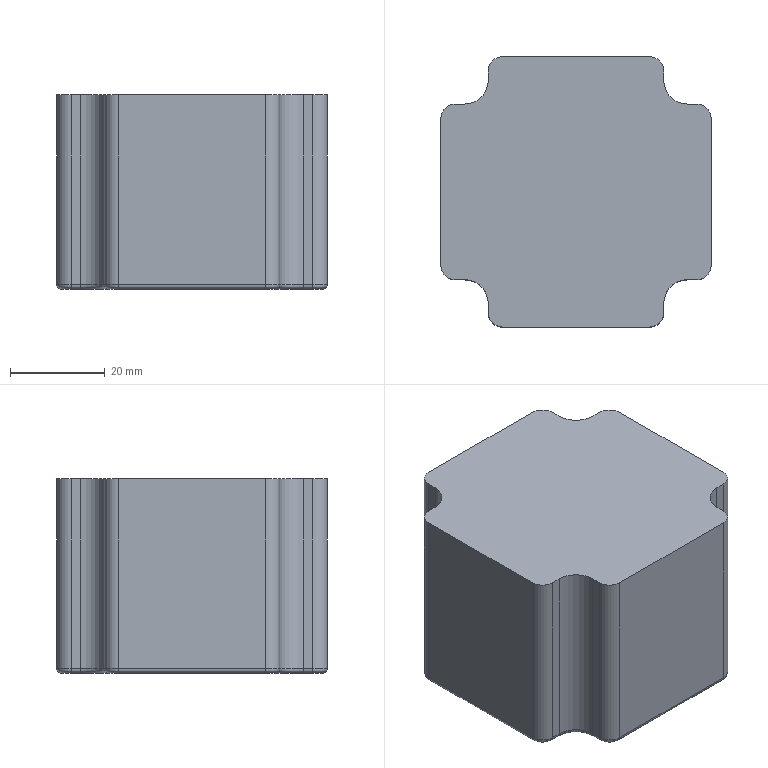Part | SolidWorks | features BaseBody 1 | 1 solid | 50 faces | box 57 x 57 x 41 mm | volume 117011 mm3 | cylinder 24 | plane 14 | torus 12 | commonest cylinder face diameters 2 x12 6 x8 10 x4
STEP:
#1=CARTESIAN_POINT('',(-18.5,23.5,41.));
#2=VERTEX_POINT('',#1);
#3=CARTESIAN_POINT('',(-18.5,23.5,1.));
#4=VERTEX_POINT('',#3);
#5=CARTESIAN_POINT('',(-18.5,23.5,41.));
#6=DIRECTION('',(0.,0.,-1.));
#7=VECTOR('',#6,1000.);
#8=LINE('',#5,#7);
#9=EDGE_CURVE('',#2,#4,#8,.T.);
#10=ORIENTED_EDGE('',*,*,#9,.T.);
#11=CARTESIAN_POINT('',(-23.5,18.5,1.));
#12=VERTEX_POINT('',#11);
#13=CARTESIAN_POINT('',(-23.5,23.5,1.));
#14=DIRECTION('',(0.,0.,-1.));
#15=DIRECTION('',(1.,0.,0.));
#16=AXIS2_PLACEMENT_3D('',#13,#14,#15);
#17=CIRCLE('',#16,5.);
#18=EDGE_CURVE('',#4,#12,#17,.T.);
#19=ORIENTED_EDGE('',*,*,#18,.T.);
#20=CARTESIAN_POINT('',(-23.5,18.5,41.));
#21=VERTEX_POINT('',#20);
#22=CARTESIAN_POINT('',(-23.5,18.5,41.));
#23=DIRECTION('',(0.,0.,-1.));
#24=VECTOR('',#23,1000.);
#25=LINE('',#22,#24);
#26=EDGE_CURVE('',#21,#12,#25,.T.);
#27=ORIENTED_EDGE('',*,*,#26,.F.);
#28=CARTESIAN_POINT('',(-23.5,23.5,41.));
#29=DIRECTION('',(0.,0.,-1.));
#30=DIRECTION('',(1.,0.,0.));
#31=AXIS2_PLACEMENT_3D('',#28,#29,#30);
#32=CIRCLE('',#31,5.);
#33=EDGE_CURVE('',#2,#21,#32,.T.);
#34=ORIENTED_EDGE('',*,*,#33,.F.);
#35=EDGE_LOOP('',(#10,#19,#27,#34));
#36=FACE_OUTER_BOUND('',#35,.T.);
#37=CARTESIAN_POINT('',(-23.5,23.5,41.));
#38=DIRECTION('',(0.,0.,-1.));
#39=DIRECTION('',(-1.,0.,0.));
#40=AXIS2_PLACEMENT_3D('',#37,#38,#39);
#41=CYLINDRICAL_SURFACE('',#40,5.);
#42=ADVANCED_FACE('',(#36),#41,.F.);
#43=ORIENTED_EDGE('',*,*,#26,.T.);
#44=CARTESIAN_POINT('',(-25.5,18.5,1.));
#45=VERTEX_POINT('',#44);
#46=CARTESIAN_POINT('',(-25.5,18.5,1.));
#47=DIRECTION('',(-1.,0.,0.));
#48=VECTOR('',#47,1000.);
#49=LINE('',#46,#48);
#50=EDGE_CURVE('',#12,#45,#49,.T.);
#51=ORIENTED_EDGE('',*,*,#50,.T.);
#52=CARTESIAN_POINT('',(-25.5,18.5,41.));
#53=VERTEX_POINT('',#52);
#54=CARTESIAN_POINT('',(-25.5,18.5,41.));
#55=DIRECTION('',(0.,0.,-1.));
#56=VECTOR('',#55,1000.);
#57=LINE('',#54,#56);
#58=EDGE_CURVE('',#53,#45,#57,.T.);
#59=ORIENTED_EDGE('',*,*,#58,.F.);
#60=CARTESIAN_POINT('',(-25.5,18.5,41.));
#61=DIRECTION('',(-1.,0.,0.));
#62=VECTOR('',#61,1000.);
#63=LINE('',#60,#62);
#64=EDGE_CURVE('',#21,#53,#63,.T.);
#65=ORIENTED_EDGE('',*,*,#64,.F.);
#66=EDGE_LOOP('',(#43,#51,#59,#65));
#67=FACE_OUTER_BOUND('',#66,.T.);
#68=CARTESIAN_POINT('',(-25.5,18.5,41.));
#69=DIRECTION('',(0.,-1.,0.));
#70=DIRECTION('',(0.,0.,-1.));
#71=AXIS2_PLACEMENT_3D('',#68,#69,#70);
#72=PLANE('',#71);
#73=ADVANCED_FACE('',(#67),#72,.F.);
#74=ORIENTED_EDGE('',*,*,#58,.T.);
#75=CARTESIAN_POINT('',(-28.5,15.5,1.));
#76=VERTEX_POINT('',#75);
#77=CARTESIAN_POINT('',(-25.5,15.5,1.));
#78=DIRECTION('',(0.,0.,1.));
#79=DIRECTION('',(1.,0.,0.));
#80=AXIS2_PLACEMENT_3D('',#77,#78,#79);
#81=CIRCLE('',#80,3.);
#82=EDGE_CURVE('',#45,#76,#81,.T.);
#83=ORIENTED_EDGE('',*,*,#82,.T.);
#84=CARTESIAN_POINT('',(-28.5,15.5,41.));
#85=VERTEX_POINT('',#84);
#86=CARTESIAN_POINT('',(-28.5,15.5,41.));
#87=DIRECTION('',(0.,0.,-1.));
#88=VECTOR('',#87,1000.);
#89=LINE('',#86,#88);
#90=EDGE_CURVE('',#85,#76,#89,.T.);
#91=ORIENTED_EDGE('',*,*,#90,.F.);
#92=CARTESIAN_POINT('',(-25.5,15.5,41.));
#93=DIRECTION('',(0.,0.,1.));
#94=DIRECTION('',(-1.,0.,0.));
#95=AXIS2_PLACEMENT_3D('',#92,#93,#94);
#96=CIRCLE('',#95,3.);
#97=EDGE_CURVE('',#53,#85,#96,.T.);
#98=ORIENTED_EDGE('',*,*,#97,.F.);
#99=EDGE_LOOP('',(#74,#83,#91,#98));
#100=FACE_OUTER_BOUND('',#99,.T.);
#101=CARTESIAN_POINT('',(-25.5,15.5,41.));
#102=DIRECTION('',(0.,0.,-1.));
#103=DIRECTION('',(-1.,0.,0.));
#104=AXIS2_PLACEMENT_3D('',#101,#102,#103);
#105=CYLINDRICAL_SURFACE('',#104,3.);
#106=ADVANCED_FACE('',(#100),#105,.T.);
#107=ORIENTED_EDGE('',*,*,#90,.T.);
#108=CARTESIAN_POINT('',(-28.5,-15.5,1.));
#109=VERTEX_POINT('',#108);
#110=CARTESIAN_POINT('',(-28.5,-15.5,1.));
#111=DIRECTION('',(0.,-1.,0.));
#112=VECTOR('',#111,1000.);
#113=LINE('',#110,#112);
#114=EDGE_CURVE('',#76,#109,#113,.T.);
#115=ORIENTED_EDGE('',*,*,#114,.T.);
#116=CARTESIAN_POINT('',(-28.5,-15.5,41.));
#117=VERTEX_POINT('',#116);
#118=CARTESIAN_POINT('',(-28.5,-15.5,41.));
#119=DIRECTION('',(0.,0.,-1.));
#120=VECTOR('',#119,1000.);
#121=LINE('',#118,#120);
#122=EDGE_CURVE('',#117,#109,#121,.T.);
#123=ORIENTED_EDGE('',*,*,#122,.F.);
#124=CARTESIAN_POINT('',(-28.5,-15.5,41.));
#125=DIRECTION('',(0.,-1.,0.));
#126=VECTOR('',#125,1000.);
#127=LINE('',#124,#126);
#128=EDGE_CURVE('',#85,#117,#127,.T.);
#129=ORIENTED_EDGE('',*,*,#128,.F.);
#130=EDGE_LOOP('',(#107,#115,#123,#129));
#131=FACE_OUTER_BOUND('',#130,.T.);
#132=CARTESIAN_POINT('',(-28.5,-15.5,41.));
#133=DIRECTION('',(1.,0.,0.));
#134=DIRECTION('',(0.,1.,0.));
#135=AXIS2_PLACEMENT_3D('',#132,#133,#134);
#136=PLANE('',#135);
#137=ADVANCED_FACE('',(#131),#136,.F.);
#138=ORIENTED_EDGE('',*,*,#122,.T.);
#139=CARTESIAN_POINT('',(-25.5,-18.5,1.));
#140=VERTEX_POINT('',#139);
#141=CARTESIAN_POINT('',(-25.5,-15.5,1.));
#142=DIRECTION('',(0.,0.,1.));
#143=DIRECTION('',(1.,0.,0.));
#144=AXIS2_PLACEMENT_3D('',#141,#142,#143);
#145=CIRCLE('',#144,3.);
#146=EDGE_CURVE('',#109,#140,#145,.T.);
#147=ORIENTED_EDGE('',*,*,#146,.T.);
#148=CARTESIAN_POINT('',(-25.5,-18.5,41.));
#149=VERTEX_POINT('',#148);
#150=CARTESIAN_POINT('',(-25.5,-18.5,41.));
#151=DIRECTION('',(0.,0.,-1.));
#152=VECTOR('',#151,1000.);
#153=LINE('',#150,#152);
#154=EDGE_CURVE('',#149,#140,#153,.T.);
#155=ORIENTED_EDGE('',*,*,#154,.F.);
#156=CARTESIAN_POINT('',(-25.5,-15.5,41.));
#157=DIRECTION('',(0.,0.,1.));
#158=DIRECTION('',(-1.,0.,0.));
#159=AXIS2_PLACEMENT_3D('',#156,#157,#158);
#160=CIRCLE('',#159,3.);
#161=EDGE_CURVE('',#117,#149,#160,.T.);
#162=ORIENTED_EDGE('',*,*,#161,.F.);
#163=EDGE_LOOP('',(#138,#147,#155,#162));
#164=FACE_OUTER_BOUND('',#163,.T.);
#165=CARTESIAN_POINT('',(-25.5,-15.5,41.));
#166=DIRECTION('',(0.,0.,-1.));
#167=DIRECTION('',(-1.,0.,0.));
#168=AXIS2_PLACEMENT_3D('',#165,#166,#167);
#169=CYLINDRICAL_SURFACE('',#168,3.);
#170=ADVANCED_FACE('',(#164),#169,.T.);
#171=ORIENTED_EDGE('',*,*,#154,.T.);
#172=CARTESIAN_POINT('',(-23.5,-18.5,1.));
#173=VERTEX_POINT('',#172);
#174=CARTESIAN_POINT('',(-25.5,-18.5,1.));
#175=DIRECTION('',(1.,0.,0.));
#176=VECTOR('',#175,1000.);
#177=LINE('',#174,#176);
#178=EDGE_CURVE('',#140,#173,#177,.T.);
#179=ORIENTED_EDGE('',*,*,#178,.T.);
#180=CARTESIAN_POINT('',(-23.5,-18.5,41.));
#181=VERTEX_POINT('',#180);
#182=CARTESIAN_POINT('',(-23.5,-18.5,41.));
#183=DIRECTION('',(0.,0.,-1.));
#184=VECTOR('',#183,1000.);
#185=LINE('',#182,#184);
#186=EDGE_CURVE('',#181,#173,#185,.T.);
#187=ORIENTED_EDGE('',*,*,#186,.F.);
#188=CARTESIAN_POINT('',(-25.5,-18.5,41.));
#189=DIRECTION('',(1.,0.,0.));
#190=VECTOR('',#189,1000.);
#191=LINE('',#188,#190);
#192=EDGE_CURVE('',#149,#181,#191,.T.);
#193=ORIENTED_EDGE('',*,*,#192,.F.);
#194=EDGE_LOOP('',(#171,#179,#187,#193));
#195=FACE_OUTER_BOUND('',#194,.T.);
#196=CARTESIAN_POINT('',(-25.5,-18.5,41.));
#197=DIRECTION('',(0.,1.,0.));
#198=DIRECTION('',(1.,0.,0.));
#199=AXIS2_PLACEMENT_3D('',#196,#197,#198);
#200=PLANE('',#199);
#201=ADVANCED_FACE('',(#195),#200,.F.);
#202=ORIENTED_EDGE('',*,*,#186,.T.);
#203=CARTESIAN_POINT('',(-18.5,-23.5,1.));
#204=VERTEX_POINT('',#203);
#205=CARTESIAN_POINT('',(-23.5,-23.5,1.));
#206=DIRECTION('',(0.,0.,-1.));
#207=DIRECTION('',(1.,0.,0.));
#208=AXIS2_PLACEMENT_3D('',#205,#206,#207);
#209=CIRCLE('',#208,5.);
#210=EDGE_CURVE('',#173,#204,#209,.T.);
#211=ORIENTED_EDGE('',*,*,#210,.T.);
#212=CARTESIAN_POINT('',(-18.5,-23.5,41.));
#213=VERTEX_POINT('',#212);
#214=CARTESIAN_POINT('',(-18.5,-23.5,41.));
#215=DIRECTION('',(0.,0.,-1.));
#216=VECTOR('',#215,1000.);
#217=LINE('',#214,#216);
#218=EDGE_CURVE('',#213,#204,#217,.T.);
#219=ORIENTED_EDGE('',*,*,#218,.F.);
#220=CARTESIAN_POINT('',(-23.5,-23.5,41.));
#221=DIRECTION('',(0.,0.,-1.));
#222=DIRECTION('',(1.,0.,0.));
#223=AXIS2_PLACEMENT_3D('',#220,#221,#222);
#224=CIRCLE('',#223,5.);
#225=EDGE_CURVE('',#181,#213,#224,.T.);
#226=ORIENTED_EDGE('',*,*,#225,.F.);
#227=EDGE_LOOP('',(#202,#211,#219,#226));
#228=FACE_OUTER_BOUND('',#227,.T.);
#229=CARTESIAN_POINT('',(-23.5,-23.5,41.));
#230=DIRECTION('',(0.,0.,-1.));
#231=DIRECTION('',(-1.,0.,0.));
#232=AXIS2_PLACEMENT_3D('',#229,#230,#231);
#233=CYLINDRICAL_SURFACE('',#232,5.);
#234=ADVANCED_FACE('',(#228),#233,.F.);
#235=ORIENTED_EDGE('',*,*,#218,.T.);
#236=CARTESIAN_POINT('',(-18.5,-25.5,1.));
#237=VERTEX_POINT('',#236);
#238=CARTESIAN_POINT('',(-18.5,-25.5,1.));
#239=DIRECTION('',(0.,-1.,0.));
#240=VECTOR('',#239,1000.);
#241=LINE('',#238,#240);
#242=EDGE_CURVE('',#204,#237,#241,.T.);
#243=ORIENTED_EDGE('',*,*,#242,.T.);
#244=CARTESIAN_POINT('',(-18.5,-25.5,41.));
#245=VERTEX_POINT('',#244);
#246=CARTESIAN_POINT('',(-18.5,-25.5,41.));
#247=DIRECTION('',(0.,0.,-1.));
#248=VECTOR('',#247,1000.);
#249=LINE('',#246,#248);
#250=EDGE_CURVE('',#245,#237,#249,.T.);
#251=ORIENTED_EDGE('',*,*,#250,.F.);
#252=CARTESIAN_POINT('',(-18.5,-25.5,41.));
#253=DIRECTION('',(0.,-1.,0.));
#254=VECTOR('',#253,1000.);
#255=LINE('',#252,#254);
#256=EDGE_CURVE('',#213,#245,#255,.T.);
#257=ORIENTED_EDGE('',*,*,#256,.F.);
#258=EDGE_LOOP('',(#235,#243,#251,#257));
#259=FACE_OUTER_BOUND('',#258,.T.);
#260=CARTESIAN_POINT('',(-18.5,-25.5,41.));
#261=DIRECTION('',(1.,0.,0.));
#262=DIRECTION('',(0.,1.,0.));
#263=AXIS2_PLACEMENT_3D('',#260,#261,#262);
#264=PLANE('',#263);
#265=ADVANCED_FACE('',(#259),#264,.F.);
#266=ORIENTED_EDGE('',*,*,#250,.T.);
#267=CARTESIAN_POINT('',(-15.5,-28.5,1.));
#268=VERTEX_POINT('',#267);
#269=CARTESIAN_POINT('',(-15.5,-25.5,1.));
#270=DIRECTION('',(0.,0.,1.));
#271=DIRECTION('',(1.,0.,0.));
#272=AXIS2_PLACEMENT_3D('',#269,#270,#271);
#273=CIRCLE('',#272,3.);
#274=EDGE_CURVE('',#237,#268,#273,.T.);
#275=ORIENTED_EDGE('',*,*,#274,.T.);
#276=CARTESIAN_POINT('',(-15.5,-28.5,41.));
#277=VERTEX_POINT('',#276);
#278=CARTESIAN_POINT('',(-15.5,-28.5,41.));
#279=DIRECTION('',(0.,0.,-1.));
#280=VECTOR('',#279,1000.);
#281=LINE('',#278,#280);
#282=EDGE_CURVE('',#277,#268,#281,.T.);
#283=ORIENTED_EDGE('',*,*,#282,.F.);
#284=CARTESIAN_POINT('',(-15.5,-25.5,41.));
#285=DIRECTION('',(0.,0.,1.));
#286=DIRECTION('',(-1.,0.,0.));
#287=AXIS2_PLACEMENT_3D('',#284,#285,#286);
#288=CIRCLE('',#287,3.);
#289=EDGE_CURVE('',#245,#277,#288,.T.);
#290=ORIENTED_EDGE('',*,*,#289,.F.);
#291=EDGE_LOOP('',(#266,#275,#283,#290));
#292=FACE_OUTER_BOUND('',#291,.T.);
#293=CARTESIAN_POINT('',(-15.5,-25.5,41.));
#294=DIRECTION('',(0.,0.,-1.));
#295=DIRECTION('',(-1.,0.,0.));
#296=AXIS2_PLACEMENT_3D('',#293,#294,#295);
#297=CYLINDRICAL_SURFACE('',#296,3.);
#298=ADVANCED_FACE('',(#292),#297,.T.);
#299=ORIENTED_EDGE('',*,*,#282,.T.);
#300=CARTESIAN_POINT('',(15.5,-28.5,1.));
#301=VERTEX_POINT('',#300);
#302=CARTESIAN_POINT('',(-15.5,-28.5,1.));
#303=DIRECTION('',(1.,0.,0.));
#304=VECTOR('',#303,1000.);
#305=LINE('',#302,#304);
#306=EDGE_CURVE('',#268,#301,#305,.T.);
#307=ORIENTED_EDGE('',*,*,#306,.T.);
#308=CARTESIAN_POINT('',(15.5,-28.5,41.));
#309=VERTEX_POINT('',#308);
#310=CARTESIAN_POINT('',(15.5,-28.5,41.));
#311=DIRECTION('',(0.,0.,-1.));
#312=VECTOR('',#311,1000.);
#313=LINE('',#310,#312);
#314=EDGE_CURVE('',#309,#301,#313,.T.);
#315=ORIENTED_EDGE('',*,*,#314,.F.);
#316=CARTESIAN_POINT('',(-15.5,-28.5,41.));
#317=DIRECTION('',(1.,0.,0.));
#318=VECTOR('',#317,1000.);
#319=LINE('',#316,#318);
#320=EDGE_CURVE('',#277,#309,#319,.T.);
#321=ORIENTED_EDGE('',*,*,#320,.F.);
#322=EDGE_LOOP('',(#299,#307,#315,#321));
#323=FACE_OUTER_BOUND('',#322,.T.);
#324=CARTESIAN_POINT('',(-15.5,-28.5,41.));
#325=DIRECTION('',(0.,1.,0.));
#326=DIRECTION('',(1.,0.,0.));
#327=AXIS2_PLACEMENT_3D('',#324,#325,#326);
#328=PLANE('',#327);
#329=ADVANCED_FACE('',(#323),#328,.F.);
#330=ORIENTED_EDGE('',*,*,#314,.T.);
#331=CARTESIAN_POINT('',(18.5,-25.5,1.));
#332=VERTEX_POINT('',#331);
#333=CARTESIAN_POINT('',(15.5,-25.5,1.));
#334=DIRECTION('',(0.,0.,1.));
#335=DIRECTION('',(1.,0.,0.));
#336=AXIS2_PLACEMENT_3D('',#333,#334,#335);
#337=CIRCLE('',#336,3.);
#338=EDGE_CURVE('',#301,#332,#337,.T.);
#339=ORIENTED_EDGE('',*,*,#338,.T.);
#340=CARTESIAN_POINT('',(18.5,-25.5,41.));
#341=VERTEX_POINT('',#340);
#342=CARTESIAN_POINT('',(18.5,-25.5,41.));
#343=DIRECTION('',(0.,0.,-1.));
#344=VECTOR('',#343,1000.);
#345=LINE('',#342,#344);
#346=EDGE_CURVE('',#341,#332,#345,.T.);
#347=ORIENTED_EDGE('',*,*,#346,.F.);
#348=CARTESIAN_POINT('',(15.5,-25.5,41.));
#349=DIRECTION('',(0.,0.,1.));
#350=DIRECTION('',(1.,0.,0.));
#351=AXIS2_PLACEMENT_3D('',#348,#349,#350);
#352=CIRCLE('',#351,3.);
#353=EDGE_CURVE('',#309,#341,#352,.T.);
#354=ORIENTED_EDGE('',*,*,#353,.F.);
#355=EDGE_LOOP('',(#330,#339,#347,#354));
#356=FACE_OUTER_BOUND('',#355,.T.);
#357=CARTESIAN_POINT('',(15.5,-25.5,41.));
#358=DIRECTION('',(0.,0.,-1.));
#359=DIRECTION('',(-1.,0.,0.));
#360=AXIS2_PLACEMENT_3D('',#357,#358,#359);
#361=CYLINDRICAL_SURFACE('',#360,3.);
#362=ADVANCED_FACE('',(#356),#361,.T.);
#363=ORIENTED_EDGE('',*,*,#346,.T.);
#364=CARTESIAN_POINT('',(18.5,-23.5,1.));
#365=VERTEX_POINT('',#364);
#366=CARTESIAN_POINT('',(18.5,-25.5,1.));
#367=DIRECTION('',(0.,1.,0.));
#368=VECTOR('',#367,1000.);
#369=LINE('',#366,#368);
#370=EDGE_CURVE('',#332,#365,#369,.T.);
#371=ORIENTED_EDGE('',*,*,#370,.T.);
#372=CARTESIAN_POINT('',(18.5,-23.5,41.));
#373=VERTEX_POINT('',#372);
#374=CARTESIAN_POINT('',(18.5,-23.5,41.));
#375=DIRECTION('',(0.,0.,-1.));
#376=VECTOR('',#375,1000.);
#377=LINE('',#374,#376);
#378=EDGE_CURVE('',#373,#365,#377,.T.);
#379=ORIENTED_EDGE('',*,*,#378,.F.);
#380=CARTESIAN_POINT('',(18.5,-25.5,41.));
#381=DIRECTION('',(0.,1.,0.));
#382=VECTOR('',#381,1000.);
#383=LINE('',#380,#382);
#384=EDGE_CURVE('',#341,#373,#383,.T.);
#385=ORIENTED_EDGE('',*,*,#384,.F.);
#386=EDGE_LOOP('',(#363,#371,#379,#385));
#387=FACE_OUTER_BOUND('',#386,.T.);
#388=CARTESIAN_POINT('',(18.5,-25.5,41.));
#389=DIRECTION('',(-1.,0.,0.));
#390=DIRECTION('',(0.,0.,1.));
#391=AXIS2_PLACEMENT_3D('',#388,#389,#390);
#392=PLANE('',#391);
#393=ADVANCED_FACE('',(#387),#392,.F.);
#394=ORIENTED_EDGE('',*,*,#378,.T.);
#395=CARTESIAN_POINT('',(23.5,-18.5,1.));
#396=VERTEX_POINT('',#395);
#397=CARTESIAN_POINT('',(23.5,-23.5,1.));
#398=DIRECTION('',(0.,0.,-1.));
#399=DIRECTION('',(1.,0.,0.));
#400=AXIS2_PLACEMENT_3D('',#397,#398,#399);
#401=CIRCLE('',#400,5.);
#402=EDGE_CURVE('',#365,#396,#401,.T.);
#403=ORIENTED_EDGE('',*,*,#402,.T.);
#404=CARTESIAN_POINT('',(23.5,-18.5,41.));
#405=VERTEX_POINT('',#404);
#406=CARTESIAN_POINT('',(23.5,-18.5,41.));
#407=DIRECTION('',(0.,0.,-1.));
#408=VECTOR('',#407,1000.);
#409=LINE('',#406,#408);
#410=EDGE_CURVE('',#405,#396,#409,.T.);
#411=ORIENTED_EDGE('',*,*,#410,.F.);
#412=CARTESIAN_POINT('',(23.5,-23.5,41.));
#413=DIRECTION('',(0.,0.,-1.));
#414=DIRECTION('',(1.,0.,0.));
#415=AXIS2_PLACEMENT_3D('',#412,#413,#414);
#416=CIRCLE('',#415,5.);
#417=EDGE_CURVE('',#373,#405,#416,.T.);
#418=ORIENTED_EDGE('',*,*,#417,.F.);
#419=EDGE_LOOP('',(#394,#403,#411,#418));
#420=FACE_OUTER_BOUND('',#419,.T.);
#421=CARTESIAN_POINT('',(23.5,-23.5,41.));
#422=DIRECTION('',(0.,0.,-1.));
#423=DIRECTION('',(-1.,0.,0.));
#424=AXIS2_PLACEMENT_3D('',#421,#422,#423);
#425=CYLINDRICAL_SURFACE('',#424,5.);
#426=ADVANCED_FACE('',(#420),#425,.F.);
#427=ORIENTED_EDGE('',*,*,#410,.T.);
#428=CARTESIAN_POINT('',(25.5,-18.5,1.));
#429=VERTEX_POINT('',#428);
#430=CARTESIAN_POINT('',(25.5,-18.5,1.));
#431=DIRECTION('',(1.,0.,0.));
#432=VECTOR('',#431,1000.);
#433=LINE('',#430,#432);
#434=EDGE_CURVE('',#396,#429,#433,.T.);
#435=ORIENTED_EDGE('',*,*,#434,.T.);
#436=CARTESIAN_POINT('',(25.5,-18.5,41.));
#437=VERTEX_POINT('',#436);
#438=CARTESIAN_POINT('',(25.5,-18.5,41.));
#439=DIRECTION('',(0.,0.,-1.));
#440=VECTOR('',#439,1000.);
#441=LINE('',#438,#440);
#442=EDGE_CURVE('',#437,#429,#441,.T.);
#443=ORIENTED_EDGE('',*,*,#442,.F.);
#444=CARTESIAN_POINT('',(25.5,-18.5,41.));
#445=DIRECTION('',(1.,0.,0.));
#446=VECTOR('',#445,1000.);
#447=LINE('',#444,#446);
#448=EDGE_CURVE('',#405,#437,#447,.T.);
#449=ORIENTED_EDGE('',*,*,#448,.F.);
#450=EDGE_LOOP('',(#427,#435,#443,#449));
#451=FACE_OUTER_BOUND('',#450,.T.);
#452=CARTESIAN_POINT('',(25.5,-18.5,41.));
#453=DIRECTION('',(0.,1.,0.));
#454=DIRECTION('',(1.,0.,0.));
#455=AXIS2_PLACEMENT_3D('',#452,#453,#454);
#456=PLANE('',#455);
#457=ADVANCED_FACE('',(#451),#456,.F.);
#458=ORIENTED_EDGE('',*,*,#442,.T.);
#459=CARTESIAN_POINT('',(28.5,-15.5,1.));
#460=VERTEX_POINT('',#459);
#461=CARTESIAN_POINT('',(25.5,-15.5,1.));
#462=DIRECTION('',(0.,0.,1.));
#463=DIRECTION('',(1.,0.,0.));
#464=AXIS2_PLACEMENT_3D('',#461,#462,#463);
#465=CIRCLE('',#464,3.);
#466=EDGE_CURVE('',#429,#460,#465,.T.);
#467=ORIENTED_EDGE('',*,*,#466,.T.);
#468=CARTESIAN_POINT('',(28.5,-15.5,41.));
#469=VERTEX_POINT('',#468);
#470=CARTESIAN_POINT('',(28.5,-15.5,41.));
#471=DIRECTION('',(0.,0.,-1.));
#472=VECTOR('',#471,1000.);
#473=LINE('',#470,#472);
#474=EDGE_CURVE('',#469,#460,#473,.T.);
#475=ORIENTED_EDGE('',*,*,#474,.F.);
#476=CARTESIAN_POINT('',(25.5,-15.5,41.));
#477=DIRECTION('',(0.,0.,1.));
#478=DIRECTION('',(-1.,0.,0.));
#479=AXIS2_PLACEMENT_3D('',#476,#477,#478);
#480=CIRCLE('',#479,3.);
#481=EDGE_CURVE('',#437,#469,#480,.T.);
#482=ORIENTED_EDGE('',*,*,#481,.F.);
#483=EDGE_LOOP('',(#458,#467,#475,#482));
#484=FACE_OUTER_BOUND('',#483,.T.);
#485=CARTESIAN_POINT('',(25.5,-15.5,41.));
#486=DIRECTION('',(0.,0.,-1.));
#487=DIRECTION('',(-1.,0.,0.));
#488=AXIS2_PLACEMENT_3D('',#485,#486,#487);
#489=CYLINDRICAL_SURFACE('',#488,3.);
#490=ADVANCED_FACE('',(#484),#489,.T.);
#491=ORIENTED_EDGE('',*,*,#474,.T.);
#492=CARTESIAN_POINT('',(28.5,15.5,1.));
#493=VERTEX_POINT('',#492);
#494=CARTESIAN_POINT('',(28.5,-15.5,1.));
#495=DIRECTION('',(0.,1.,0.));
#496=VECTOR('',#495,1000.);
#497=LINE('',#494,#496);
#498=EDGE_CURVE('',#460,#493,#497,.T.);
#499=ORIENTED_EDGE('',*,*,#498,.T.);
#500=CARTESIAN_POINT('',(28.5,15.5,41.));
#501=VERTEX_POINT('',#500);
#502=CARTESIAN_POINT('',(28.5,15.5,41.));
#503=DIRECTION('',(0.,0.,-1.));
#504=VECTOR('',#503,1000.);
#505=LINE('',#502,#504);
#506=EDGE_CURVE('',#501,#493,#505,.T.);
#507=ORIENTED_EDGE('',*,*,#506,.F.);
#508=CARTESIAN_POINT('',(28.5,-15.5,41.));
#509=DIRECTION('',(0.,1.,0.));
#510=VECTOR('',#509,1000.);
#511=LINE('',#508,#510);
#512=EDGE_CURVE('',#469,#501,#511,.T.);
#513=ORIENTED_EDGE('',*,*,#512,.F.);
#514=EDGE_LOOP('',(#491,#499,#507,#513));
#515=FACE_OUTER_BOUND('',#514,.T.);
#516=CARTESIAN_POINT('',(28.5,-15.5,41.));
#517=DIRECTION('',(-1.,0.,0.));
#518=DIRECTION('',(0.,0.,1.));
#519=AXIS2_PLACEMENT_3D('',#516,#517,#518);
#520=PLANE('',#519);
#521=ADVANCED_FACE('',(#515),#520,.F.);
#522=ORIENTED_EDGE('',*,*,#506,.T.);
#523=CARTESIAN_POINT('',(25.5,18.5,1.));
#524=VERTEX_POINT('',#523);
#525=CARTESIAN_POINT('',(25.5,15.5,1.));
#526=DIRECTION('',(0.,0.,1.));
#527=DIRECTION('',(1.,0.,0.));
#528=AXIS2_PLACEMENT_3D('',#525,#526,#527);
#529=CIRCLE('',#528,3.);
#530=EDGE_CURVE('',#493,#524,#529,.T.);
#531=ORIENTED_EDGE('',*,*,#530,.T.);
#532=CARTESIAN_POINT('',(25.5,18.5,41.));
#533=VERTEX_POINT('',#532);
#534=CARTESIAN_POINT('',(25.5,18.5,41.));
#535=DIRECTION('',(0.,0.,-1.));
#536=VECTOR('',#535,1000.);
#537=LINE('',#534,#536);
#538=EDGE_CURVE('',#533,#524,#537,.T.);
#539=ORIENTED_EDGE('',*,*,#538,.F.);
#540=CARTESIAN_POINT('',(25.5,15.5,41.));
#541=DIRECTION('',(0.,0.,1.));
#542=DIRECTION('',(1.,0.,0.));
#543=AXIS2_PLACEMENT_3D('',#540,#541,#542);
#544=CIRCLE('',#543,3.);
#545=EDGE_CURVE('',#501,#533,#544,.T.);
#546=ORIENTED_EDGE('',*,*,#545,.F.);
#547=EDGE_LOOP('',(#522,#531,#539,#546));
#548=FACE_OUTER_BOUND('',#547,.T.);
#549=CARTESIAN_POINT('',(25.5,15.5,41.));
#550=DIRECTION('',(0.,0.,-1.));
#551=DIRECTION('',(-1.,0.,0.));
#552=AXIS2_PLACEMENT_3D('',#549,#550,#551);
#553=CYLINDRICAL_SURFACE('',#552,3.);
#554=ADVANCED_FACE('',(#548),#553,.T.);
#555=ORIENTED_EDGE('',*,*,#538,.T.);
#556=CARTESIAN_POINT('',(23.5,18.5,1.));
#557=VERTEX_POINT('',#556);
#558=CARTESIAN_POINT('',(25.5,18.5,1.));
#559=DIRECTION('',(-1.,0.,0.));
#560=VECTOR('',#559,1000.);
#561=LINE('',#558,#560);
#562=EDGE_CURVE('',#524,#557,#561,.T.);
#563=ORIENTED_EDGE('',*,*,#562,.T.);
#564=CARTESIAN_POINT('',(23.5,18.5,41.));
#565=VERTEX_POINT('',#564);
#566=CARTESIAN_POINT('',(23.5,18.5,41.));
#567=DIRECTION('',(0.,0.,-1.));
#568=VECTOR('',#567,1000.);
#569=LINE('',#566,#568);
#570=EDGE_CURVE('',#565,#557,#569,.T.);
#571=ORIENTED_EDGE('',*,*,#570,.F.);
#572=CARTESIAN_POINT('',(25.5,18.5,41.));
#573=DIRECTION('',(-1.,0.,0.));
#574=VECTOR('',#573,1000.);
#575=LINE('',#572,#574);
#576=EDGE_CURVE('',#533,#565,#575,.T.);
#577=ORIENTED_EDGE('',*,*,#576,.F.);
#578=EDGE_LOOP('',(#555,#563,#571,#577));
#579=FACE_OUTER_BOUND('',#578,.T.);
#580=CARTESIAN_POINT('',(25.5,18.5,41.));
#581=DIRECTION('',(0.,-1.,0.));
#582=DIRECTION('',(0.,0.,-1.));
#583=AXIS2_PLACEMENT_3D('',#580,#581,#582);
#584=PLANE('',#583);
#585=ADVANCED_FACE('',(#579),#584,.F.);
#586=ORIENTED_EDGE('',*,*,#570,.T.);
#587=CARTESIAN_POINT('',(18.5,23.5,1.));
#588=VERTEX_POINT('',#587);
#589=CARTESIAN_POINT('',(23.5,23.5,1.));
#590=DIRECTION('',(0.,0.,-1.));
#591=DIRECTION('',(1.,0.,0.));
#592=AXIS2_PLACEMENT_3D('',#589,#590,#591);
#593=CIRCLE('',#592,5.);
#594=EDGE_CURVE('',#557,#588,#593,.T.);
#595=ORIENTED_EDGE('',*,*,#594,.T.);
#596=CARTESIAN_POINT('',(18.5,23.5,41.));
#597=VERTEX_POINT('',#596);
#598=CARTESIAN_POINT('',(18.5,23.5,41.));
#599=DIRECTION('',(0.,0.,-1.));
#600=VECTOR('',#599,1000.);
#601=LINE('',#598,#600);
#602=EDGE_CURVE('',#597,#588,#601,.T.);
#603=ORIENTED_EDGE('',*,*,#602,.F.);
#604=CARTESIAN_POINT('',(23.5,23.5,41.));
#605=DIRECTION('',(0.,0.,-1.));
#606=DIRECTION('',(1.,0.,0.));
#607=AXIS2_PLACEMENT_3D('',#604,#605,#606);
#608=CIRCLE('',#607,5.);
#609=EDGE_CURVE('',#565,#597,#608,.T.);
#610=ORIENTED_EDGE('',*,*,#609,.F.);
#611=EDGE_LOOP('',(#586,#595,#603,#610));
#612=FACE_OUTER_BOUND('',#611,.T.);
#613=CARTESIAN_POINT('',(23.5,23.5,41.));
#614=DIRECTION('',(0.,0.,-1.));
#615=DIRECTION('',(-1.,0.,0.));
#616=AXIS2_PLACEMENT_3D('',#613,#614,#615);
#617=CYLINDRICAL_SURFACE('',#616,5.);
#618=ADVANCED_FACE('',(#612),#617,.F.);
#619=ORIENTED_EDGE('',*,*,#602,.T.);
#620=CARTESIAN_POINT('',(18.5,25.5,1.));
#621=VERTEX_POINT('',#620);
#622=CARTESIAN_POINT('',(18.5,25.5,1.));
#623=DIRECTION('',(0.,1.,0.));
#624=VECTOR('',#623,1000.);
#625=LINE('',#622,#624);
#626=EDGE_CURVE('',#588,#621,#625,.T.);
#627=ORIENTED_EDGE('',*,*,#626,.T.);
#628=CARTESIAN_POINT('',(18.5,25.5,41.));
#629=VERTEX_POINT('',#628);
#630=CARTESIAN_POINT('',(18.5,25.5,41.));
#631=DIRECTION('',(0.,0.,-1.));
#632=VECTOR('',#631,1000.);
#633=LINE('',#630,#632);
#634=EDGE_CURVE('',#629,#621,#633,.T.);
#635=ORIENTED_EDGE('',*,*,#634,.F.);
#636=CARTESIAN_POINT('',(18.5,25.5,41.));
#637=DIRECTION('',(0.,1.,0.));
#638=VECTOR('',#637,1000.);
#639=LINE('',#636,#638);
#640=EDGE_CURVE('',#597,#629,#639,.T.);
#641=ORIENTED_EDGE('',*,*,#640,.F.);
#642=EDGE_LOOP('',(#619,#627,#635,#641));
#643=FACE_OUTER_BOUND('',#642,.T.);
#644=CARTESIAN_POINT('',(18.5,25.5,41.));
#645=DIRECTION('',(-1.,0.,0.));
#646=DIRECTION('',(0.,1.,0.));
#647=AXIS2_PLACEMENT_3D('',#644,#645,#646);
#648=PLANE('',#647);
#649=ADVANCED_FACE('',(#643),#648,.F.);
#650=ORIENTED_EDGE('',*,*,#634,.T.);
#651=CARTESIAN_POINT('',(15.5,28.5,1.));
#652=VERTEX_POINT('',#651);
#653=CARTESIAN_POINT('',(15.5,25.5,1.));
#654=DIRECTION('',(0.,0.,1.));
#655=DIRECTION('',(1.,0.,0.));
#656=AXIS2_PLACEMENT_3D('',#653,#654,#655);
#657=CIRCLE('',#656,3.);
#658=EDGE_CURVE('',#621,#652,#657,.T.);
#659=ORIENTED_EDGE('',*,*,#658,.T.);
#660=CARTESIAN_POINT('',(15.5,28.5,41.));
#661=VERTEX_POINT('',#660);
#662=CARTESIAN_POINT('',(15.5,28.5,41.));
#663=DIRECTION('',(0.,0.,-1.));
#664=VECTOR('',#663,1000.);
#665=LINE('',#662,#664);
#666=EDGE_CURVE('',#661,#652,#665,.T.);
#667=ORIENTED_EDGE('',*,*,#666,.F.);
#668=CARTESIAN_POINT('',(15.5,25.5,41.));
#669=DIRECTION('',(0.,0.,1.));
#670=DIRECTION('',(1.,0.,0.));
#671=AXIS2_PLACEMENT_3D('',#668,#669,#670);
#672=CIRCLE('',#671,3.);
#673=EDGE_CURVE('',#629,#661,#672,.T.);
#674=ORIENTED_EDGE('',*,*,#673,.F.);
#675=EDGE_LOOP('',(#650,#659,#667,#674));
#676=FACE_OUTER_BOUND('',#675,.T.);
#677=CARTESIAN_POINT('',(15.5,25.5,41.));
#678=DIRECTION('',(0.,0.,-1.));
#679=DIRECTION('',(-1.,0.,0.));
#680=AXIS2_PLACEMENT_3D('',#677,#678,#679);
#681=CYLINDRICAL_SURFACE('',#680,3.);
#682=ADVANCED_FACE('',(#676),#681,.T.);
#683=ORIENTED_EDGE('',*,*,#666,.T.);
#684=CARTESIAN_POINT('',(-15.5,28.5,1.));
#685=VERTEX_POINT('',#684);
#686=CARTESIAN_POINT('',(-15.5,28.5,1.));
#687=DIRECTION('',(-1.,0.,0.));
#688=VECTOR('',#687,1000.);
#689=LINE('',#686,#688);
#690=EDGE_CURVE('',#652,#685,#689,.T.);
#691=ORIENTED_EDGE('',*,*,#690,.T.);
#692=CARTESIAN_POINT('',(-15.5,28.5,41.));
#693=VERTEX_POINT('',#692);
#694=CARTESIAN_POINT('',(-15.5,28.5,41.));
#695=DIRECTION('',(0.,0.,-1.));
#696=VECTOR('',#695,1000.);
#697=LINE('',#694,#696);
#698=EDGE_CURVE('',#693,#685,#697,.T.);
#699=ORIENTED_EDGE('',*,*,#698,.F.);
#700=CARTESIAN_POINT('',(-15.5,28.5,41.));
#701=DIRECTION('',(-1.,0.,0.));
#702=VECTOR('',#701,1000.);
#703=LINE('',#700,#702);
#704=EDGE_CURVE('',#661,#693,#703,.T.);
#705=ORIENTED_EDGE('',*,*,#704,.F.);
#706=EDGE_LOOP('',(#683,#691,#699,#705));
#707=FACE_OUTER_BOUND('',#706,.T.);
#708=CARTESIAN_POINT('',(-15.5,28.5,41.));
#709=DIRECTION('',(0.,-1.,0.));
#710=DIRECTION('',(0.,0.,-1.));
#711=AXIS2_PLACEMENT_3D('',#708,#709,#710);
#712=PLANE('',#711);
#713=ADVANCED_FACE('',(#707),#712,.F.);
#714=ORIENTED_EDGE('',*,*,#698,.T.);
#715=CARTESIAN_POINT('',(-18.5,25.5,1.));
#716=VERTEX_POINT('',#715);
#717=CARTESIAN_POINT('',(-15.5,25.5,1.));
#718=DIRECTION('',(0.,0.,1.));
#719=DIRECTION('',(1.,0.,0.));
#720=AXIS2_PLACEMENT_3D('',#717,#718,#719);
#721=CIRCLE('',#720,3.);
#722=EDGE_CURVE('',#685,#716,#721,.T.);
#723=ORIENTED_EDGE('',*,*,#722,.T.);
#724=CARTESIAN_POINT('',(-18.5,25.5,41.));
#725=VERTEX_POINT('',#724);
#726=CARTESIAN_POINT('',(-18.5,25.5,41.));
#727=DIRECTION('',(0.,0.,-1.));
#728=VECTOR('',#727,1000.);
#729=LINE('',#726,#728);
#730=EDGE_CURVE('',#725,#716,#729,.T.);
#731=ORIENTED_EDGE('',*,*,#730,.F.);
#732=CARTESIAN_POINT('',(-15.5,25.5,41.));
#733=DIRECTION('',(0.,0.,1.));
#734=DIRECTION('',(-1.,0.,0.));
#735=AXIS2_PLACEMENT_3D('',#732,#733,#734);
#736=CIRCLE('',#735,3.);
#737=EDGE_CURVE('',#693,#725,#736,.T.);
#738=ORIENTED_EDGE('',*,*,#737,.F.);
#739=EDGE_LOOP('',(#714,#723,#731,#738));
#740=FACE_OUTER_BOUND('',#739,.T.);
#741=CARTESIAN_POINT('',(-15.5,25.5,41.));
#742=DIRECTION('',(0.,0.,-1.));
#743=DIRECTION('',(-1.,0.,0.));
#744=AXIS2_PLACEMENT_3D('',#741,#742,#743);
#745=CYLINDRICAL_SURFACE('',#744,3.);
#746=ADVANCED_FACE('',(#740),#745,.T.);
#747=ORIENTED_EDGE('',*,*,#730,.T.);
#748=CARTESIAN_POINT('',(-18.5,25.5,1.));
#749=DIRECTION('',(0.,-1.,0.));
#750=VECTOR('',#749,1000.);
#751=LINE('',#748,#750);
#752=EDGE_CURVE('',#716,#4,#751,.T.);
#753=ORIENTED_EDGE('',*,*,#752,.T.);
#754=ORIENTED_EDGE('',*,*,#9,.F.);
#755=CARTESIAN_POINT('',(-18.5,25.5,41.));
#756=DIRECTION('',(0.,-1.,0.));
#757=VECTOR('',#756,1000.);
#758=LINE('',#755,#757);
#759=EDGE_CURVE('',#725,#2,#758,.T.);
#760=ORIENTED_EDGE('',*,*,#759,.F.);
#761=EDGE_LOOP('',(#747,#753,#754,#760));
#762=FACE_OUTER_BOUND('',#761,.T.);
#763=CARTESIAN_POINT('',(-18.5,25.5,41.));
#764=DIRECTION('',(1.,0.,0.));
#765=DIRECTION('',(0.,-1.,0.));
#766=AXIS2_PLACEMENT_3D('',#763,#764,#765);
#767=PLANE('',#766);
#768=ADVANCED_FACE('',(#762),#767,.F.);
#769=ORIENTED_EDGE('',*,*,#33,.T.);
#770=ORIENTED_EDGE('',*,*,#64,.T.);
#771=ORIENTED_EDGE('',*,*,#97,.T.);
#772=ORIENTED_EDGE('',*,*,#128,.T.);
#773=ORIENTED_EDGE('',*,*,#161,.T.);
#774=ORIENTED_EDGE('',*,*,#192,.T.);
#775=ORIENTED_EDGE('',*,*,#225,.T.);
#776=ORIENTED_EDGE('',*,*,#256,.T.);
#777=ORIENTED_EDGE('',*,*,#289,.T.);
#778=ORIENTED_EDGE('',*,*,#320,.T.);
#779=ORIENTED_EDGE('',*,*,#353,.T.);
#780=ORIENTED_EDGE('',*,*,#384,.T.);
#781=ORIENTED_EDGE('',*,*,#417,.T.);
#782=ORIENTED_EDGE('',*,*,#448,.T.);
#783=ORIENTED_EDGE('',*,*,#481,.T.);
#784=ORIENTED_EDGE('',*,*,#512,.T.);
#785=ORIENTED_EDGE('',*,*,#545,.T.);
#786=ORIENTED_EDGE('',*,*,#576,.T.);
#787=ORIENTED_EDGE('',*,*,#609,.T.);
#788=ORIENTED_EDGE('',*,*,#640,.T.);
#789=ORIENTED_EDGE('',*,*,#673,.T.);
#790=ORIENTED_EDGE('',*,*,#704,.T.);
#791=ORIENTED_EDGE('',*,*,#737,.T.);
#792=ORIENTED_EDGE('',*,*,#759,.T.);
#793=EDGE_LOOP('',(#769,#770,#771,#772,#773,#774,#775,#776,#777,#778,#779,#780,#781,#782,#783,#784,#785,#786,#787,#788,#789,#790,#791,#792));
#794=FACE_OUTER_BOUND('',#793,.T.);
#795=CARTESIAN_POINT('',(-23.5,23.5,41.));
#796=DIRECTION('',(0.,0.,1.));
#797=DIRECTION('',(1.,0.,0.));
#798=AXIS2_PLACEMENT_3D('',#795,#796,#797);
#799=PLANE('',#798);
#800=ADVANCED_FACE('',(#794),#799,.T.);
#801=CARTESIAN_POINT('',(-27.5,15.5,0.));
#802=VERTEX_POINT('',#801);
#803=CARTESIAN_POINT('',(-25.5,17.5,0.));
#804=VERTEX_POINT('',#803);
#805=CARTESIAN_POINT('',(-25.5,15.5,0.));
#806=DIRECTION('',(0.,0.,-1.));
#807=DIRECTION('',(1.,0.,0.));
#808=AXIS2_PLACEMENT_3D('',#805,#806,#807);
#809=CIRCLE('',#808,2.);
#810=EDGE_CURVE('',#802,#804,#809,.T.);
#811=ORIENTED_EDGE('',*,*,#810,.T.);
#812=CARTESIAN_POINT('',(-23.5,17.5,0.));
#813=VERTEX_POINT('',#812);
#814=CARTESIAN_POINT('',(-23.5,17.5,0.));
#815=DIRECTION('',(1.,0.,0.));
#816=VECTOR('',#815,1000.);
#817=LINE('',#814,#816);
#818=EDGE_CURVE('',#804,#813,#817,.T.);
#819=ORIENTED_EDGE('',*,*,#818,.T.);
#820=CARTESIAN_POINT('',(-17.5,23.5,0.));
#821=VERTEX_POINT('',#820);
#822=CARTESIAN_POINT('',(-23.5,23.5,0.));
#823=DIRECTION('',(0.,0.,1.));
#824=DIRECTION('',(1.,0.,0.));
#825=AXIS2_PLACEMENT_3D('',#822,#823,#824);
#826=CIRCLE('',#825,6.);
#827=EDGE_CURVE('',#813,#821,#826,.T.);
#828=ORIENTED_EDGE('',*,*,#827,.T.);
#829=CARTESIAN_POINT('',(-17.5,25.5,0.));
#830=VERTEX_POINT('',#829);
#831=CARTESIAN_POINT('',(-17.5,23.5,0.));
#832=DIRECTION('',(0.,1.,0.));
#833=VECTOR('',#832,1000.);
#834=LINE('',#831,#833);
#835=EDGE_CURVE('',#821,#830,#834,.T.);
#836=ORIENTED_EDGE('',*,*,#835,.T.);
#837=CARTESIAN_POINT('',(-15.5,27.5,0.));
#838=VERTEX_POINT('',#837);
#839=CARTESIAN_POINT('',(-15.5,25.5,0.));
#840=DIRECTION('',(0.,0.,-1.));
#841=DIRECTION('',(1.,0.,0.));
#842=AXIS2_PLACEMENT_3D('',#839,#840,#841);
#843=CIRCLE('',#842,2.);
#844=EDGE_CURVE('',#830,#838,#843,.T.);
#845=ORIENTED_EDGE('',*,*,#844,.T.);
#846=CARTESIAN_POINT('',(15.5,27.5,0.));
#847=VERTEX_POINT('',#846);
#848=CARTESIAN_POINT('',(-23.5,27.5,0.));
#849=DIRECTION('',(1.,0.,0.));
#850=VECTOR('',#849,1000.);
#851=LINE('',#848,#850);
#852=EDGE_CURVE('',#838,#847,#851,.T.);
#853=ORIENTED_EDGE('',*,*,#852,.T.);
#854=CARTESIAN_POINT('',(17.5,25.5,0.));
#855=VERTEX_POINT('',#854);
#856=CARTESIAN_POINT('',(15.5,25.5,0.));
#857=DIRECTION('',(0.,0.,-1.));
#858=DIRECTION('',(1.,0.,0.));
#859=AXIS2_PLACEMENT_3D('',#856,#857,#858);
#860=CIRCLE('',#859,2.);
#861=EDGE_CURVE('',#847,#855,#860,.T.);
#862=ORIENTED_EDGE('',*,*,#861,.T.);
#863=CARTESIAN_POINT('',(17.5,23.5,0.));
#864=VERTEX_POINT('',#863);
#865=CARTESIAN_POINT('',(17.5,23.5,0.));
#866=DIRECTION('',(0.,-1.,0.));
#867=VECTOR('',#866,1000.);
#868=LINE('',#865,#867);
#869=EDGE_CURVE('',#855,#864,#868,.T.);
#870=ORIENTED_EDGE('',*,*,#869,.T.);
#871=CARTESIAN_POINT('',(23.5,17.5,0.));
#872=VERTEX_POINT('',#871);
#873=CARTESIAN_POINT('',(23.5,23.5,0.));
#874=DIRECTION('',(0.,0.,1.));
#875=DIRECTION('',(1.,0.,0.));
#876=AXIS2_PLACEMENT_3D('',#873,#874,#875);
#877=CIRCLE('',#876,6.);
#878=EDGE_CURVE('',#864,#872,#877,.T.);
#879=ORIENTED_EDGE('',*,*,#878,.T.);
#880=CARTESIAN_POINT('',(25.5,17.5,0.));
#881=VERTEX_POINT('',#880);
#882=CARTESIAN_POINT('',(-23.5,17.5,0.));
#883=DIRECTION('',(1.,0.,0.));
#884=VECTOR('',#883,1000.);
#885=LINE('',#882,#884);
#886=EDGE_CURVE('',#872,#881,#885,.T.);
#887=ORIENTED_EDGE('',*,*,#886,.T.);
#888=CARTESIAN_POINT('',(27.5,15.5,0.));
#889=VERTEX_POINT('',#888);
#890=CARTESIAN_POINT('',(25.5,15.5,0.));
#891=DIRECTION('',(0.,0.,-1.));
#892=DIRECTION('',(1.,0.,0.));
#893=AXIS2_PLACEMENT_3D('',#890,#891,#892);
#894=CIRCLE('',#893,2.);
#895=EDGE_CURVE('',#881,#889,#894,.T.);
#896=ORIENTED_EDGE('',*,*,#895,.T.);
#897=CARTESIAN_POINT('',(27.5,-15.5,0.));
#898=VERTEX_POINT('',#897);
#899=CARTESIAN_POINT('',(27.5,23.5,0.));
#900=DIRECTION('',(0.,-1.,0.));
#901=VECTOR('',#900,1000.);
#902=LINE('',#899,#901);
#903=EDGE_CURVE('',#889,#898,#902,.T.);
#904=ORIENTED_EDGE('',*,*,#903,.T.);
#905=CARTESIAN_POINT('',(25.5,-17.5,0.));
#906=VERTEX_POINT('',#905);
#907=CARTESIAN_POINT('',(25.5,-15.5,0.));
#908=DIRECTION('',(0.,0.,-1.));
#909=DIRECTION('',(1.,0.,0.));
#910=AXIS2_PLACEMENT_3D('',#907,#908,#909);
#911=CIRCLE('',#910,2.);
#912=EDGE_CURVE('',#898,#906,#911,.T.);
#913=ORIENTED_EDGE('',*,*,#912,.T.);
#914=CARTESIAN_POINT('',(23.5,-17.5,0.));
#915=VERTEX_POINT('',#914);
#916=CARTESIAN_POINT('',(-23.5,-17.5,0.));
#917=DIRECTION('',(-1.,0.,0.));
#918=VECTOR('',#917,1000.);
#919=LINE('',#916,#918);
#920=EDGE_CURVE('',#906,#915,#919,.T.);
#921=ORIENTED_EDGE('',*,*,#920,.T.);
#922=CARTESIAN_POINT('',(17.5,-23.5,0.));
#923=VERTEX_POINT('',#922);
#924=CARTESIAN_POINT('',(23.5,-23.5,0.));
#925=DIRECTION('',(0.,0.,1.));
#926=DIRECTION('',(1.,0.,0.));
#927=AXIS2_PLACEMENT_3D('',#924,#925,#926);
#928=CIRCLE('',#927,6.);
#929=EDGE_CURVE('',#915,#923,#928,.T.);
#930=ORIENTED_EDGE('',*,*,#929,.T.);
#931=CARTESIAN_POINT('',(17.5,-25.5,0.));
#932=VERTEX_POINT('',#931);
#933=CARTESIAN_POINT('',(17.5,23.5,0.));
#934=DIRECTION('',(0.,-1.,0.));
#935=VECTOR('',#934,1000.);
#936=LINE('',#933,#935);
#937=EDGE_CURVE('',#923,#932,#936,.T.);
#938=ORIENTED_EDGE('',*,*,#937,.T.);
#939=CARTESIAN_POINT('',(15.5,-27.5,0.));
#940=VERTEX_POINT('',#939);
#941=CARTESIAN_POINT('',(15.5,-25.5,0.));
#942=DIRECTION('',(0.,0.,-1.));
#943=DIRECTION('',(1.,0.,0.));
#944=AXIS2_PLACEMENT_3D('',#941,#942,#943);
#945=CIRCLE('',#944,2.);
#946=EDGE_CURVE('',#932,#940,#945,.T.);
#947=ORIENTED_EDGE('',*,*,#946,.T.);
#948=CARTESIAN_POINT('',(-15.5,-27.5,0.));
#949=VERTEX_POINT('',#948);
#950=CARTESIAN_POINT('',(-23.5,-27.5,0.));
#951=DIRECTION('',(-1.,0.,0.));
#952=VECTOR('',#951,1000.);
#953=LINE('',#950,#952);
#954=EDGE_CURVE('',#940,#949,#953,.T.);
#955=ORIENTED_EDGE('',*,*,#954,.T.);
#956=CARTESIAN_POINT('',(-17.5,-25.5,0.));
#957=VERTEX_POINT('',#956);
#958=CARTESIAN_POINT('',(-15.5,-25.5,0.));
#959=DIRECTION('',(0.,0.,-1.));
#960=DIRECTION('',(1.,0.,0.));
#961=AXIS2_PLACEMENT_3D('',#958,#959,#960);
#962=CIRCLE('',#961,2.);
#963=EDGE_CURVE('',#949,#957,#962,.T.);
#964=ORIENTED_EDGE('',*,*,#963,.T.);
#965=CARTESIAN_POINT('',(-17.5,-23.5,0.));
#966=VERTEX_POINT('',#965);
#967=CARTESIAN_POINT('',(-17.5,23.5,0.));
#968=DIRECTION('',(0.,1.,0.));
#969=VECTOR('',#968,1000.);
#970=LINE('',#967,#969);
#971=EDGE_CURVE('',#957,#966,#970,.T.);
#972=ORIENTED_EDGE('',*,*,#971,.T.);
#973=CARTESIAN_POINT('',(-23.5,-17.5,0.));
#974=VERTEX_POINT('',#973);
#975=CARTESIAN_POINT('',(-23.5,-23.5,0.));
#976=DIRECTION('',(0.,0.,1.));
#977=DIRECTION('',(1.,0.,0.));
#978=AXIS2_PLACEMENT_3D('',#975,#976,#977);
#979=CIRCLE('',#978,6.);
#980=EDGE_CURVE('',#966,#974,#979,.T.);
#981=ORIENTED_EDGE('',*,*,#980,.T.);
#982=CARTESIAN_POINT('',(-25.5,-17.5,0.));
#983=VERTEX_POINT('',#982);
#984=CARTESIAN_POINT('',(-23.5,-17.5,0.));
#985=DIRECTION('',(-1.,0.,0.));
#986=VECTOR('',#985,1000.);
#987=LINE('',#984,#986);
#988=EDGE_CURVE('',#974,#983,#987,.T.);
#989=ORIENTED_EDGE('',*,*,#988,.T.);
#990=CARTESIAN_POINT('',(-27.5,-15.5,0.));
#991=VERTEX_POINT('',#990);
#992=CARTESIAN_POINT('',(-25.5,-15.5,0.));
#993=DIRECTION('',(0.,0.,-1.));
#994=DIRECTION('',(1.,0.,0.));
#995=AXIS2_PLACEMENT_3D('',#992,#993,#994);
#996=CIRCLE('',#995,2.);
#997=EDGE_CURVE('',#983,#991,#996,.T.);
#998=ORIENTED_EDGE('',*,*,#997,.T.);
#999=CARTESIAN_POINT('',(-27.5,23.5,0.));
#1000=DIRECTION('',(0.,1.,0.));
#1001=VECTOR('',#1000,1000.);
#1002=LINE('',#999,#1001);
#1003=EDGE_CURVE('',#991,#802,#1002,.T.);
#1004=ORIENTED_EDGE('',*,*,#1003,.T.);
#1005=EDGE_LOOP('',(#811,#819,#828,#836,#845,#853,#862,#870,#879,#887,#896,#904,#913,#921,#930,#938,#947,#955,#964,#972,#981,#989,#998,#1004));
#1006=FACE_OUTER_BOUND('',#1005,.T.);
#1007=CARTESIAN_POINT('',(-23.5,23.5,0.));
#1008=DIRECTION('',(0.,0.,1.));
#1009=DIRECTION('',(1.,0.,0.));
#1010=AXIS2_PLACEMENT_3D('',#1007,#1008,#1009);
#1011=PLANE('',#1010);
#1012=ADVANCED_FACE('',(#1006),#1011,.F.);
#1013=CARTESIAN_POINT('',(23.5,-17.5,1.));
#1014=DIRECTION('',(-1.,0.,0.));
#1015=DIRECTION('',(0.,0.,1.));
#1016=AXIS2_PLACEMENT_3D('',#1013,#1014,#1015);
#1017=CIRCLE('',#1016,1.);
#1018=EDGE_CURVE('',#915,#396,#1017,.T.);
#1019=ORIENTED_EDGE('',*,*,#1018,.F.);
#1020=ORIENTED_EDGE('',*,*,#920,.F.);
#1021=CARTESIAN_POINT('',(25.5,-17.5,1.));
#1022=DIRECTION('',(1.,0.,0.));
#1023=DIRECTION('',(0.,0.,-1.));
#1024=AXIS2_PLACEMENT_3D('',#1021,#1022,#1023);
#1025=CIRCLE('',#1024,1.);
#1026=EDGE_CURVE('',#429,#906,#1025,.T.);
#1027=ORIENTED_EDGE('',*,*,#1026,.F.);
#1028=ORIENTED_EDGE('',*,*,#434,.F.);
#1029=EDGE_LOOP('',(#1019,#1020,#1027,#1028));
#1030=FACE_OUTER_BOUND('',#1029,.T.);
#1031=CARTESIAN_POINT('',(25.5,-17.5,1.));
#1032=DIRECTION('',(1.,0.,0.));
#1033=DIRECTION('',(0.,0.,-1.));
#1034=AXIS2_PLACEMENT_3D('',#1031,#1032,#1033);
#1035=CYLINDRICAL_SURFACE('',#1034,1.);
#1036=ADVANCED_FACE('',(#1030),#1035,.T.);
#1037=ORIENTED_EDGE('',*,*,#1026,.T.);
#1038=ORIENTED_EDGE('',*,*,#912,.F.);
#1039=CARTESIAN_POINT('',(27.5,-15.5,1.));
#1040=DIRECTION('',(0.,1.,0.));
#1041=DIRECTION('',(0.,0.,1.));
#1042=AXIS2_PLACEMENT_3D('',#1039,#1040,#1041);
#1043=CIRCLE('',#1042,1.);
#1044=EDGE_CURVE('',#460,#898,#1043,.T.);
#1045=ORIENTED_EDGE('',*,*,#1044,.F.);
#1046=ORIENTED_EDGE('',*,*,#466,.F.);
#1047=EDGE_LOOP('',(#1037,#1038,#1045,#1046));
#1048=FACE_OUTER_BOUND('',#1047,.T.);
#1049=CARTESIAN_POINT('',(25.5,-15.5,1.));
#1050=DIRECTION('',(0.,0.,1.));
#1051=DIRECTION('',(1.,0.,0.));
#1052=AXIS2_PLACEMENT_3D('',#1049,#1050,#1051);
#1053=TOROIDAL_SURFACE('',#1052,2.,1.);
#1054=ADVANCED_FACE('',(#1048),#1053,.T.);
#1055=ORIENTED_EDGE('',*,*,#1018,.T.);
#1056=ORIENTED_EDGE('',*,*,#402,.F.);
#1057=CARTESIAN_POINT('',(17.5,-23.5,1.));
#1058=DIRECTION('',(0.,-1.,0.));
#1059=DIRECTION('',(1.,0.,0.));
#1060=AXIS2_PLACEMENT_3D('',#1057,#1058,#1059);
#1061=CIRCLE('',#1060,1.);
#1062=EDGE_CURVE('',#923,#365,#1061,.T.);
#1063=ORIENTED_EDGE('',*,*,#1062,.F.);
#1064=ORIENTED_EDGE('',*,*,#929,.F.);
#1065=EDGE_LOOP('',(#1055,#1056,#1063,#1064));
#1066=FACE_OUTER_BOUND('',#1065,.T.);
#1067=CARTESIAN_POINT('',(23.5,-23.5,1.));
#1068=DIRECTION('',(0.,0.,1.));
#1069=DIRECTION('',(1.,0.,0.));
#1070=AXIS2_PLACEMENT_3D('',#1067,#1068,#1069);
#1071=TOROIDAL_SURFACE('',#1070,6.,1.);
#1072=ADVANCED_FACE('',(#1066),#1071,.T.);
#1073=ORIENTED_EDGE('',*,*,#1044,.T.);
#1074=ORIENTED_EDGE('',*,*,#903,.F.);
#1075=CARTESIAN_POINT('',(27.5,15.5,1.));
#1076=DIRECTION('',(0.,1.,0.));
#1077=DIRECTION('',(0.,0.,1.));
#1078=AXIS2_PLACEMENT_3D('',#1075,#1076,#1077);
#1079=CIRCLE('',#1078,1.);
#1080=EDGE_CURVE('',#493,#889,#1079,.T.);
#1081=ORIENTED_EDGE('',*,*,#1080,.F.);
#1082=ORIENTED_EDGE('',*,*,#498,.F.);
#1083=EDGE_LOOP('',(#1073,#1074,#1081,#1082));
#1084=FACE_OUTER_BOUND('',#1083,.T.);
#1085=CARTESIAN_POINT('',(27.5,-15.5,1.));
#1086=DIRECTION('',(0.,1.,0.));
#1087=DIRECTION('',(0.,0.,1.));
#1088=AXIS2_PLACEMENT_3D('',#1085,#1086,#1087);
#1089=CYLINDRICAL_SURFACE('',#1088,1.);
#1090=ADVANCED_FACE('',(#1084),#1089,.T.);
#1091=ORIENTED_EDGE('',*,*,#1062,.T.);
#1092=ORIENTED_EDGE('',*,*,#370,.F.);
#1093=CARTESIAN_POINT('',(17.5,-25.5,1.));
#1094=DIRECTION('',(0.,-1.,0.));
#1095=DIRECTION('',(0.,0.,-1.));
#1096=AXIS2_PLACEMENT_3D('',#1093,#1094,#1095);
#1097=CIRCLE('',#1096,1.);
#1098=EDGE_CURVE('',#932,#332,#1097,.T.);
#1099=ORIENTED_EDGE('',*,*,#1098,.F.);
#1100=ORIENTED_EDGE('',*,*,#937,.F.);
#1101=EDGE_LOOP('',(#1091,#1092,#1099,#1100));
#1102=FACE_OUTER_BOUND('',#1101,.T.);
#1103=CARTESIAN_POINT('',(17.5,-25.5,1.));
#1104=DIRECTION('',(0.,1.,0.));
#1105=DIRECTION('',(-1.,0.,0.));
#1106=AXIS2_PLACEMENT_3D('',#1103,#1104,#1105);
#1107=CYLINDRICAL_SURFACE('',#1106,1.);
#1108=ADVANCED_FACE('',(#1102),#1107,.T.);
#1109=ORIENTED_EDGE('',*,*,#1080,.T.);
#1110=ORIENTED_EDGE('',*,*,#895,.F.);
#1111=CARTESIAN_POINT('',(25.5,17.5,1.));
#1112=DIRECTION('',(-1.,0.,0.));
#1113=DIRECTION('',(0.,0.,1.));
#1114=AXIS2_PLACEMENT_3D('',#1111,#1112,#1113);
#1115=CIRCLE('',#1114,1.);
#1116=EDGE_CURVE('',#524,#881,#1115,.T.);
#1117=ORIENTED_EDGE('',*,*,#1116,.F.);
#1118=ORIENTED_EDGE('',*,*,#530,.F.);
#1119=EDGE_LOOP('',(#1109,#1110,#1117,#1118));
#1120=FACE_OUTER_BOUND('',#1119,.T.);
#1121=CARTESIAN_POINT('',(25.5,15.5,1.));
#1122=DIRECTION('',(0.,0.,1.));
#1123=DIRECTION('',(1.,0.,0.));
#1124=AXIS2_PLACEMENT_3D('',#1121,#1122,#1123);
#1125=TOROIDAL_SURFACE('',#1124,2.,1.);
#1126=ADVANCED_FACE('',(#1120),#1125,.T.);
#1127=ORIENTED_EDGE('',*,*,#1098,.T.);
#1128=ORIENTED_EDGE('',*,*,#338,.F.);
#1129=CARTESIAN_POINT('',(15.5,-27.5,1.));
#1130=DIRECTION('',(-1.,0.,0.));
#1131=DIRECTION('',(0.,0.,1.));
#1132=AXIS2_PLACEMENT_3D('',#1129,#1130,#1131);
#1133=CIRCLE('',#1132,1.);
#1134=EDGE_CURVE('',#940,#301,#1133,.T.);
#1135=ORIENTED_EDGE('',*,*,#1134,.F.);
#1136=ORIENTED_EDGE('',*,*,#946,.F.);
#1137=EDGE_LOOP('',(#1127,#1128,#1135,#1136));
#1138=FACE_OUTER_BOUND('',#1137,.T.);
#1139=CARTESIAN_POINT('',(15.5,-25.5,1.));
#1140=DIRECTION('',(0.,0.,1.));
#1141=DIRECTION('',(1.,0.,0.));
#1142=AXIS2_PLACEMENT_3D('',#1139,#1140,#1141);
#1143=TOROIDAL_SURFACE('',#1142,2.,1.);
#1144=ADVANCED_FACE('',(#1138),#1143,.T.);
#1145=ORIENTED_EDGE('',*,*,#1116,.T.);
#1146=ORIENTED_EDGE('',*,*,#886,.F.);
#1147=CARTESIAN_POINT('',(23.5,17.5,1.));
#1148=DIRECTION('',(-1.,0.,0.));
#1149=DIRECTION('',(0.,0.,1.));
#1150=AXIS2_PLACEMENT_3D('',#1147,#1148,#1149);
#1151=CIRCLE('',#1150,1.);
#1152=EDGE_CURVE('',#557,#872,#1151,.T.);
#1153=ORIENTED_EDGE('',*,*,#1152,.F.);
#1154=ORIENTED_EDGE('',*,*,#562,.F.);
#1155=EDGE_LOOP('',(#1145,#1146,#1153,#1154));
#1156=FACE_OUTER_BOUND('',#1155,.T.);
#1157=CARTESIAN_POINT('',(25.5,17.5,1.));
#1158=DIRECTION('',(-1.,0.,0.));
#1159=DIRECTION('',(0.,0.,1.));
#1160=AXIS2_PLACEMENT_3D('',#1157,#1158,#1159);
#1161=CYLINDRICAL_SURFACE('',#1160,1.);
#1162=ADVANCED_FACE('',(#1156),#1161,.T.);
#1163=ORIENTED_EDGE('',*,*,#1134,.T.);
#1164=ORIENTED_EDGE('',*,*,#306,.F.);
#1165=CARTESIAN_POINT('',(-15.5,-27.5,1.));
#1166=DIRECTION('',(-1.,0.,0.));
#1167=DIRECTION('',(0.,0.,1.));
#1168=AXIS2_PLACEMENT_3D('',#1165,#1166,#1167);
#1169=CIRCLE('',#1168,1.);
#1170=EDGE_CURVE('',#949,#268,#1169,.T.);
#1171=ORIENTED_EDGE('',*,*,#1170,.F.);
#1172=ORIENTED_EDGE('',*,*,#954,.F.);
#1173=EDGE_LOOP('',(#1163,#1164,#1171,#1172));
#1174=FACE_OUTER_BOUND('',#1173,.T.);
#1175=CARTESIAN_POINT('',(-15.5,-27.5,1.));
#1176=DIRECTION('',(1.,0.,0.));
#1177=DIRECTION('',(0.,0.,-1.));
#1178=AXIS2_PLACEMENT_3D('',#1175,#1176,#1177);
#1179=CYLINDRICAL_SURFACE('',#1178,1.);
#1180=ADVANCED_FACE('',(#1174),#1179,.T.);
#1181=ORIENTED_EDGE('',*,*,#1152,.T.);
#1182=ORIENTED_EDGE('',*,*,#878,.F.);
#1183=CARTESIAN_POINT('',(17.5,23.5,1.));
#1184=DIRECTION('',(0.,1.,0.));
#1185=DIRECTION('',(0.,0.,1.));
#1186=AXIS2_PLACEMENT_3D('',#1183,#1184,#1185);
#1187=CIRCLE('',#1186,1.);
#1188=EDGE_CURVE('',#588,#864,#1187,.T.);
#1189=ORIENTED_EDGE('',*,*,#1188,.F.);
#1190=ORIENTED_EDGE('',*,*,#594,.F.);
#1191=EDGE_LOOP('',(#1181,#1182,#1189,#1190));
#1192=FACE_OUTER_BOUND('',#1191,.T.);
#1193=CARTESIAN_POINT('',(23.5,23.5,1.));
#1194=DIRECTION('',(0.,0.,1.));
#1195=DIRECTION('',(1.,0.,0.));
#1196=AXIS2_PLACEMENT_3D('',#1193,#1194,#1195);
#1197=TOROIDAL_SURFACE('',#1196,6.,1.);
#1198=ADVANCED_FACE('',(#1192),#1197,.T.);
#1199=ORIENTED_EDGE('',*,*,#1170,.T.);
#1200=ORIENTED_EDGE('',*,*,#274,.F.);
#1201=CARTESIAN_POINT('',(-17.5,-25.5,1.));
#1202=DIRECTION('',(0.,1.,0.));
#1203=DIRECTION('',(-1.,0.,0.));
#1204=AXIS2_PLACEMENT_3D('',#1201,#1202,#1203);
#1205=CIRCLE('',#1204,1.);
#1206=EDGE_CURVE('',#957,#237,#1205,.T.);
#1207=ORIENTED_EDGE('',*,*,#1206,.F.);
#1208=ORIENTED_EDGE('',*,*,#963,.F.);
#1209=EDGE_LOOP('',(#1199,#1200,#1207,#1208));
#1210=FACE_OUTER_BOUND('',#1209,.T.);
#1211=CARTESIAN_POINT('',(-15.5,-25.5,1.));
#1212=DIRECTION('',(0.,0.,1.));
#1213=DIRECTION('',(1.,0.,0.));
#1214=AXIS2_PLACEMENT_3D('',#1211,#1212,#1213);
#1215=TOROIDAL_SURFACE('',#1214,2.,1.);
#1216=ADVANCED_FACE('',(#1210),#1215,.T.);
#1217=ORIENTED_EDGE('',*,*,#1188,.T.);
#1218=ORIENTED_EDGE('',*,*,#869,.F.);
#1219=CARTESIAN_POINT('',(17.5,25.5,1.));
#1220=DIRECTION('',(0.,1.,0.));
#1221=DIRECTION('',(-1.,0.,0.));
#1222=AXIS2_PLACEMENT_3D('',#1219,#1220,#1221);
#1223=CIRCLE('',#1222,1.);
#1224=EDGE_CURVE('',#621,#855,#1223,.T.);
#1225=ORIENTED_EDGE('',*,*,#1224,.F.);
#1226=ORIENTED_EDGE('',*,*,#626,.F.);
#1227=EDGE_LOOP('',(#1217,#1218,#1225,#1226));
#1228=FACE_OUTER_BOUND('',#1227,.T.);
#1229=CARTESIAN_POINT('',(17.5,25.5,1.));
#1230=DIRECTION('',(0.,1.,0.));
#1231=DIRECTION('',(-1.,0.,0.));
#1232=AXIS2_PLACEMENT_3D('',#1229,#1230,#1231);
#1233=CYLINDRICAL_SURFACE('',#1232,1.);
#1234=ADVANCED_FACE('',(#1228),#1233,.T.);
#1235=ORIENTED_EDGE('',*,*,#1206,.T.);
#1236=ORIENTED_EDGE('',*,*,#242,.F.);
#1237=CARTESIAN_POINT('',(-17.5,-23.5,1.));
#1238=DIRECTION('',(0.,1.,0.));
#1239=DIRECTION('',(0.,0.,1.));
#1240=AXIS2_PLACEMENT_3D('',#1237,#1238,#1239);
#1241=CIRCLE('',#1240,1.);
#1242=EDGE_CURVE('',#966,#204,#1241,.T.);
#1243=ORIENTED_EDGE('',*,*,#1242,.F.);
#1244=ORIENTED_EDGE('',*,*,#971,.F.);
#1245=EDGE_LOOP('',(#1235,#1236,#1243,#1244));
#1246=FACE_OUTER_BOUND('',#1245,.T.);
#1247=CARTESIAN_POINT('',(-17.5,-25.5,1.));
#1248=DIRECTION('',(0.,-1.,0.));
#1249=DIRECTION('',(1.,0.,0.));
#1250=AXIS2_PLACEMENT_3D('',#1247,#1248,#1249);
#1251=CYLINDRICAL_SURFACE('',#1250,1.);
#1252=ADVANCED_FACE('',(#1246),#1251,.T.);
#1253=ORIENTED_EDGE('',*,*,#1224,.T.);
#1254=ORIENTED_EDGE('',*,*,#861,.F.);
#1255=CARTESIAN_POINT('',(15.5,27.5,1.));
#1256=DIRECTION('',(-1.,0.,0.));
#1257=DIRECTION('',(0.,0.,1.));
#1258=AXIS2_PLACEMENT_3D('',#1255,#1256,#1257);
#1259=CIRCLE('',#1258,1.);
#1260=EDGE_CURVE('',#652,#847,#1259,.T.);
#1261=ORIENTED_EDGE('',*,*,#1260,.F.);
#1262=ORIENTED_EDGE('',*,*,#658,.F.);
#1263=EDGE_LOOP('',(#1253,#1254,#1261,#1262));
#1264=FACE_OUTER_BOUND('',#1263,.T.);
#1265=CARTESIAN_POINT('',(15.5,25.5,1.));
#1266=DIRECTION('',(0.,0.,1.));
#1267=DIRECTION('',(1.,0.,0.));
#1268=AXIS2_PLACEMENT_3D('',#1265,#1266,#1267);
#1269=TOROIDAL_SURFACE('',#1268,2.,1.);
#1270=ADVANCED_FACE('',(#1264),#1269,.T.);
#1271=ORIENTED_EDGE('',*,*,#1242,.T.);
#1272=ORIENTED_EDGE('',*,*,#210,.F.);
#1273=CARTESIAN_POINT('',(-23.5,-17.5,1.));
#1274=DIRECTION('',(-1.,0.,0.));
#1275=DIRECTION('',(0.,0.,1.));
#1276=AXIS2_PLACEMENT_3D('',#1273,#1274,#1275);
#1277=CIRCLE('',#1276,1.);
#1278=EDGE_CURVE('',#974,#173,#1277,.T.);
#1279=ORIENTED_EDGE('',*,*,#1278,.F.);
#1280=ORIENTED_EDGE('',*,*,#980,.F.);
#1281=EDGE_LOOP('',(#1271,#1272,#1279,#1280));
#1282=FACE_OUTER_BOUND('',#1281,.T.);
#1283=CARTESIAN_POINT('',(-23.5,-23.5,1.));
#1284=DIRECTION('',(0.,0.,1.));
#1285=DIRECTION('',(1.,0.,0.));
#1286=AXIS2_PLACEMENT_3D('',#1283,#1284,#1285);
#1287=TOROIDAL_SURFACE('',#1286,6.,1.);
#1288=ADVANCED_FACE('',(#1282),#1287,.T.);
#1289=ORIENTED_EDGE('',*,*,#1260,.T.);
#1290=ORIENTED_EDGE('',*,*,#852,.F.);
#1291=CARTESIAN_POINT('',(-15.5,27.5,1.));
#1292=DIRECTION('',(-1.,0.,0.));
#1293=DIRECTION('',(0.,0.,1.));
#1294=AXIS2_PLACEMENT_3D('',#1291,#1292,#1293);
#1295=CIRCLE('',#1294,1.);
#1296=EDGE_CURVE('',#685,#838,#1295,.T.);
#1297=ORIENTED_EDGE('',*,*,#1296,.F.);
#1298=ORIENTED_EDGE('',*,*,#690,.F.);
#1299=EDGE_LOOP('',(#1289,#1290,#1297,#1298));
#1300=FACE_OUTER_BOUND('',#1299,.T.);
#1301=CARTESIAN_POINT('',(-15.5,27.5,1.));
#1302=DIRECTION('',(-1.,0.,0.));
#1303=DIRECTION('',(0.,0.,1.));
#1304=AXIS2_PLACEMENT_3D('',#1301,#1302,#1303);
#1305=CYLINDRICAL_SURFACE('',#1304,1.);
#1306=ADVANCED_FACE('',(#1300),#1305,.T.);
#1307=ORIENTED_EDGE('',*,*,#1278,.T.);
#1308=ORIENTED_EDGE('',*,*,#178,.F.);
#1309=CARTESIAN_POINT('',(-25.5,-17.5,1.));
#1310=DIRECTION('',(-1.,0.,0.));
#1311=DIRECTION('',(0.,0.,1.));
#1312=AXIS2_PLACEMENT_3D('',#1309,#1310,#1311);
#1313=CIRCLE('',#1312,1.);
#1314=EDGE_CURVE('',#983,#140,#1313,.T.);
#1315=ORIENTED_EDGE('',*,*,#1314,.F.);
#1316=ORIENTED_EDGE('',*,*,#988,.F.);
#1317=EDGE_LOOP('',(#1307,#1308,#1315,#1316));
#1318=FACE_OUTER_BOUND('',#1317,.T.);
#1319=CARTESIAN_POINT('',(-25.5,-17.5,1.));
#1320=DIRECTION('',(1.,0.,0.));
#1321=DIRECTION('',(0.,0.,-1.));
#1322=AXIS2_PLACEMENT_3D('',#1319,#1320,#1321);
#1323=CYLINDRICAL_SURFACE('',#1322,1.);
#1324=ADVANCED_FACE('',(#1318),#1323,.T.);
#1325=ORIENTED_EDGE('',*,*,#1296,.T.);
#1326=ORIENTED_EDGE('',*,*,#844,.F.);
#1327=CARTESIAN_POINT('',(-17.5,25.5,1.));
#1328=DIRECTION('',(0.,-1.,0.));
#1329=DIRECTION('',(0.,0.,-1.));
#1330=AXIS2_PLACEMENT_3D('',#1327,#1328,#1329);
#1331=CIRCLE('',#1330,1.);
#1332=EDGE_CURVE('',#716,#830,#1331,.T.);
#1333=ORIENTED_EDGE('',*,*,#1332,.F.);
#1334=ORIENTED_EDGE('',*,*,#722,.F.);
#1335=EDGE_LOOP('',(#1325,#1326,#1333,#1334));
#1336=FACE_OUTER_BOUND('',#1335,.T.);
#1337=CARTESIAN_POINT('',(-15.5,25.5,1.));
#1338=DIRECTION('',(0.,0.,1.));
#1339=DIRECTION('',(1.,0.,0.));
#1340=AXIS2_PLACEMENT_3D('',#1337,#1338,#1339);
#1341=TOROIDAL_SURFACE('',#1340,2.,1.);
#1342=ADVANCED_FACE('',(#1336),#1341,.T.);
#1343=ORIENTED_EDGE('',*,*,#1314,.T.);
#1344=ORIENTED_EDGE('',*,*,#146,.F.);
#1345=CARTESIAN_POINT('',(-27.5,-15.5,1.));
#1346=DIRECTION('',(0.,1.,0.));
#1347=DIRECTION('',(0.,0.,1.));
#1348=AXIS2_PLACEMENT_3D('',#1345,#1346,#1347);
#1349=CIRCLE('',#1348,1.);
#1350=EDGE_CURVE('',#991,#109,#1349,.T.);
#1351=ORIENTED_EDGE('',*,*,#1350,.F.);
#1352=ORIENTED_EDGE('',*,*,#997,.F.);
#1353=EDGE_LOOP('',(#1343,#1344,#1351,#1352));
#1354=FACE_OUTER_BOUND('',#1353,.T.);
#1355=CARTESIAN_POINT('',(-25.5,-15.5,1.));
#1356=DIRECTION('',(0.,0.,1.));
#1357=DIRECTION('',(1.,0.,0.));
#1358=AXIS2_PLACEMENT_3D('',#1355,#1356,#1357);
#1359=TOROIDAL_SURFACE('',#1358,2.,1.);
#1360=ADVANCED_FACE('',(#1354),#1359,.T.);
#1361=ORIENTED_EDGE('',*,*,#1332,.T.);
#1362=ORIENTED_EDGE('',*,*,#835,.F.);
#1363=CARTESIAN_POINT('',(-17.5,23.5,1.));
#1364=DIRECTION('',(0.,-1.,0.));
#1365=DIRECTION('',(1.,0.,0.));
#1366=AXIS2_PLACEMENT_3D('',#1363,#1364,#1365);
#1367=CIRCLE('',#1366,1.);
#1368=EDGE_CURVE('',#4,#821,#1367,.T.);
#1369=ORIENTED_EDGE('',*,*,#1368,.F.);
#1370=ORIENTED_EDGE('',*,*,#752,.F.);
#1371=EDGE_LOOP('',(#1361,#1362,#1369,#1370));
#1372=FACE_OUTER_BOUND('',#1371,.T.);
#1373=CARTESIAN_POINT('',(-17.5,25.5,1.));
#1374=DIRECTION('',(0.,-1.,0.));
#1375=DIRECTION('',(1.,0.,0.));
#1376=AXIS2_PLACEMENT_3D('',#1373,#1374,#1375);
#1377=CYLINDRICAL_SURFACE('',#1376,1.);
#1378=ADVANCED_FACE('',(#1372),#1377,.T.);
#1379=ORIENTED_EDGE('',*,*,#1350,.T.);
#1380=ORIENTED_EDGE('',*,*,#114,.F.);
#1381=CARTESIAN_POINT('',(-27.5,15.5,1.));
#1382=DIRECTION('',(0.,1.,0.));
#1383=DIRECTION('',(0.,0.,1.));
#1384=AXIS2_PLACEMENT_3D('',#1381,#1382,#1383);
#1385=CIRCLE('',#1384,1.);
#1386=EDGE_CURVE('',#802,#76,#1385,.T.);
#1387=ORIENTED_EDGE('',*,*,#1386,.F.);
#1388=ORIENTED_EDGE('',*,*,#1003,.F.);
#1389=EDGE_LOOP('',(#1379,#1380,#1387,#1388));
#1390=FACE_OUTER_BOUND('',#1389,.T.);
#1391=CARTESIAN_POINT('',(-27.5,-15.5,1.));
#1392=DIRECTION('',(0.,-1.,0.));
#1393=DIRECTION('',(0.,0.,-1.));
#1394=AXIS2_PLACEMENT_3D('',#1391,#1392,#1393);
#1395=CYLINDRICAL_SURFACE('',#1394,1.);
#1396=ADVANCED_FACE('',(#1390),#1395,.T.);
#1397=ORIENTED_EDGE('',*,*,#1368,.T.);
#1398=ORIENTED_EDGE('',*,*,#827,.F.);
#1399=CARTESIAN_POINT('',(-23.5,17.5,1.));
#1400=DIRECTION('',(-1.,0.,0.));
#1401=DIRECTION('',(0.,0.,1.));
#1402=AXIS2_PLACEMENT_3D('',#1399,#1400,#1401);
#1403=CIRCLE('',#1402,1.);
#1404=EDGE_CURVE('',#12,#813,#1403,.T.);
#1405=ORIENTED_EDGE('',*,*,#1404,.F.);
#1406=ORIENTED_EDGE('',*,*,#18,.F.);
#1407=EDGE_LOOP('',(#1397,#1398,#1405,#1406));
#1408=FACE_OUTER_BOUND('',#1407,.T.);
#1409=CARTESIAN_POINT('',(-23.5,23.5,1.));
#1410=DIRECTION('',(0.,0.,1.));
#1411=DIRECTION('',(1.,0.,0.));
#1412=AXIS2_PLACEMENT_3D('',#1409,#1410,#1411);
#1413=TOROIDAL_SURFACE('',#1412,6.,1.);
#1414=ADVANCED_FACE('',(#1408),#1413,.T.);
#1415=ORIENTED_EDGE('',*,*,#1386,.T.);
#1416=ORIENTED_EDGE('',*,*,#82,.F.);
#1417=CARTESIAN_POINT('',(-25.5,17.5,1.));
#1418=DIRECTION('',(1.,0.,0.));
#1419=DIRECTION('',(0.,0.,-1.));
#1420=AXIS2_PLACEMENT_3D('',#1417,#1418,#1419);
#1421=CIRCLE('',#1420,1.);
#1422=EDGE_CURVE('',#804,#45,#1421,.T.);
#1423=ORIENTED_EDGE('',*,*,#1422,.F.);
#1424=ORIENTED_EDGE('',*,*,#810,.F.);
#1425=EDGE_LOOP('',(#1415,#1416,#1423,#1424));
#1426=FACE_OUTER_BOUND('',#1425,.T.);
#1427=CARTESIAN_POINT('',(-25.5,15.5,1.));
#1428=DIRECTION('',(0.,0.,1.));
#1429=DIRECTION('',(1.,0.,0.));
#1430=AXIS2_PLACEMENT_3D('',#1427,#1428,#1429);
#1431=TOROIDAL_SURFACE('',#1430,2.,1.);
#1432=ADVANCED_FACE('',(#1426),#1431,.T.);
#1433=ORIENTED_EDGE('',*,*,#1404,.T.);
#1434=ORIENTED_EDGE('',*,*,#818,.F.);
#1435=ORIENTED_EDGE('',*,*,#1422,.T.);
#1436=ORIENTED_EDGE('',*,*,#50,.F.);
#1437=EDGE_LOOP('',(#1433,#1434,#1435,#1436));
#1438=FACE_OUTER_BOUND('',#1437,.T.);
#1439=CARTESIAN_POINT('',(-25.5,17.5,1.));
#1440=DIRECTION('',(-1.,0.,0.));
#1441=DIRECTION('',(0.,0.,1.));
#1442=AXIS2_PLACEMENT_3D('',#1439,#1440,#1441);
#1443=CYLINDRICAL_SURFACE('',#1442,1.);
#1444=ADVANCED_FACE('',(#1438),#1443,.T.);
#1445=CLOSED_SHELL('',(#42,#73,#106,#137,#170,#201,#234,#265,#298,#329,#362,#393,#426,#457,#490,#521,#554,#585,#618,#649,#682,#713,#746,#768,#800,#1012,#1036,#1054,#1072,#1090,#1108,#1126,#1144,#1162,#1180,#1198,#1216,#1234,#1252,#1270,#1288,#1306,#1324,#1342,#1360,#1378,#1396,#1414,#1432,#1444));
#1446=MANIFOLD_SOLID_BREP('',#1445);
#1447=CARTESIAN_POINT('',(0.,0.,0.));
#1448=DIRECTION('',(0.,0.,1.));
#1449=DIRECTION('',(1.,0.,0.));
#1450=AXIS2_PLACEMENT_3D('',#1447,#1448,#1449);
#1451=(LENGTH_UNIT()NAMED_UNIT(*)SI_UNIT(.MILLI.,.METRE.));
#1452=UNCERTAINTY_MEASURE_WITH_UNIT(LENGTH_MEASURE(0.00001),#1451,'','');
#1453=(NAMED_UNIT(*)PLANE_ANGLE_UNIT()SI_UNIT($,.RADIAN.));
#1454=(NAMED_UNIT(*)SI_UNIT($,.STERADIAN.)SOLID_ANGLE_UNIT());
#1455=(GEOMETRIC_REPRESENTATION_CONTEXT(3)GLOBAL_UNCERTAINTY_ASSIGNED_CONTEXT((#1452))GLOBAL_UNIT_ASSIGNED_CONTEXT((#1451,#1453,#1454))REPRESENTATION_CONTEXT('',''));
#1456=ADVANCED_BREP_SHAPE_REPRESENTATION('',(#1446,#1450),#1455);